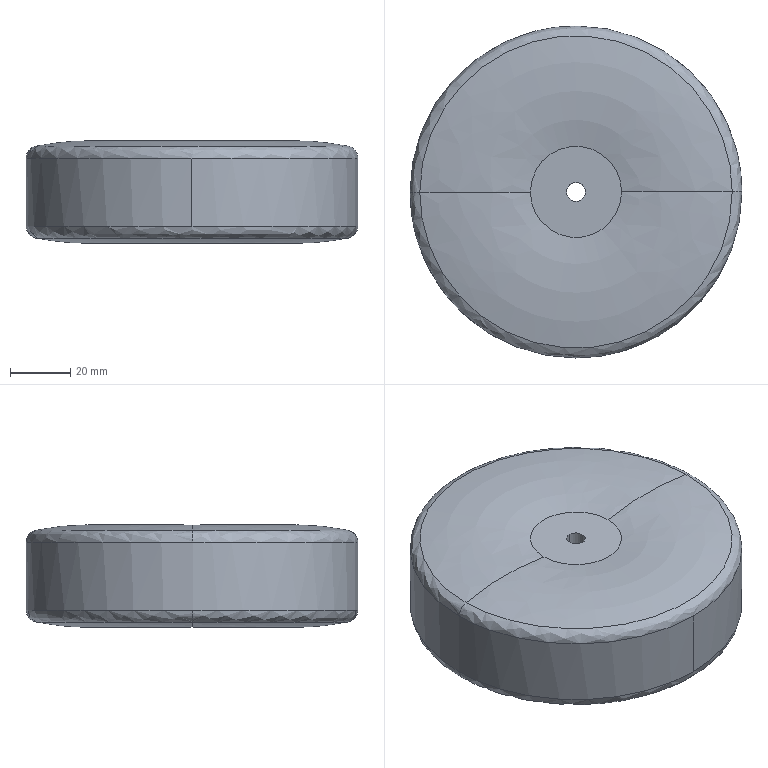Part | SolidWorks | features BaseBody 1 | 1 solid | 19 faces | box 110 x 110 x 34 mm | volume 303850 mm3 | spline 10 | cylinder 6 | plane 3 | commonest cylinder face diameters 6.2 x2 10.5 x2 110 x2
STEP:
#1=CARTESIAN_POINT('',(576.44,-187.714,1.889));
#2=VERTEX_POINT('',#1);
#3=CARTESIAN_POINT('',(606.64,-187.582,1.889));
#4=VERTEX_POINT('',#3);
#5=CARTESIAN_POINT('',(591.54,-187.648,1.889));
#6=DIRECTION('',(0.000000001,-0.000000003,1.));
#7=DIRECTION('',(0.,1.,0.000000003));
#8=AXIS2_PLACEMENT_3D('',#5,#6,#7);
#9=CIRCLE('',#8,15.1);
#10=EDGE_CURVE('',#2,#4,#9,.T.);
#11=ORIENTED_EDGE('',*,*,#10,.F.);
#12=CARTESIAN_POINT('',(539.765,-187.873,1.813));
#13=VERTEX_POINT('',#12);
#14=CARTESIAN_POINT('',(576.44,-187.714,1.889));
#15=CARTESIAN_POINT('',(573.541,-187.726,2.449));
#16=CARTESIAN_POINT('',(567.449,-187.753,3.336));
#17=CARTESIAN_POINT('',(558.099,-187.794,3.786));
#18=CARTESIAN_POINT('',(548.751,-187.834,3.297));
#19=CARTESIAN_POINT('',(542.662,-187.861,2.385));
#20=CARTESIAN_POINT('',(539.765,-187.873,1.813));
#21=B_SPLINE_CURVE_WITH_KNOTS('',3,(#14,#15,#16,#17,#18,#19,#20),.UNSPECIFIED.,.F.,.F.,(4,1,1,1,4),(0.01923,0.25,0.5,0.75,0.9808),.UNSPECIFIED.);
#22=EDGE_CURVE('',#2,#13,#21,.T.);
#23=ORIENTED_EDGE('',*,*,#22,.T.);
#24=CARTESIAN_POINT('',(643.315,-187.423,1.813));
#25=VERTEX_POINT('',#24);
#26=CARTESIAN_POINT('',(643.315,-187.423,1.813));
#27=CARTESIAN_POINT('',(643.765,-290.972,1.813));
#28=CARTESIAN_POINT('',(540.216,-291.423,1.813));
#29=CARTESIAN_POINT('',(539.765,-187.873,1.813));
#30=(BOUNDED_CURVE()B_SPLINE_CURVE(3,(#26,#27,#28,#29),.UNSPECIFIED.,.F.,.F.)B_SPLINE_CURVE_WITH_KNOTS((4,4),(0.,1.),.UNSPECIFIED.)CURVE()GEOMETRIC_REPRESENTATION_ITEM()RATIONAL_B_SPLINE_CURVE((1.,0.3333,0.3333,1.))REPRESENTATION_ITEM(''));
#31=EDGE_CURVE('',#25,#13,#30,.T.);
#32=ORIENTED_EDGE('',*,*,#31,.F.);
#33=CARTESIAN_POINT('',(606.64,-187.582,1.889));
#34=CARTESIAN_POINT('',(609.538,-187.57,2.449));
#35=CARTESIAN_POINT('',(615.631,-187.543,3.336));
#36=CARTESIAN_POINT('',(624.981,-187.503,3.786));
#37=CARTESIAN_POINT('',(634.329,-187.462,3.297));
#38=CARTESIAN_POINT('',(640.418,-187.435,2.385));
#39=CARTESIAN_POINT('',(643.315,-187.423,1.813));
#40=B_SPLINE_CURVE_WITH_KNOTS('',3,(#33,#34,#35,#36,#37,#38,#39),.UNSPECIFIED.,.F.,.F.,(4,1,1,1,4),(0.01923,0.25,0.5,0.75,0.9808),.UNSPECIFIED.);
#41=EDGE_CURVE('',#4,#25,#40,.T.);
#42=ORIENTED_EDGE('',*,*,#41,.F.);
#43=EDGE_LOOP('',(#11,#23,#32,#42));
#44=FACE_OUTER_BOUND('',#43,.T.);
#45=CARTESIAN_POINT('',(606.64,-187.582,1.889));
#46=CARTESIAN_POINT('',(606.771,-217.782,1.889));
#47=CARTESIAN_POINT('',(576.572,-217.914,1.889));
#48=CARTESIAN_POINT('',(576.44,-187.714,1.889));
#49=CARTESIAN_POINT('',(609.538,-187.57,2.449));
#50=CARTESIAN_POINT('',(609.695,-223.567,2.449));
#51=CARTESIAN_POINT('',(573.698,-223.724,2.449));
#52=CARTESIAN_POINT('',(573.541,-187.726,2.449));
#53=CARTESIAN_POINT('',(615.631,-187.543,3.336));
#54=CARTESIAN_POINT('',(615.841,-235.726,3.336));
#55=CARTESIAN_POINT('',(567.658,-235.936,3.336));
#56=CARTESIAN_POINT('',(567.449,-187.753,3.336));
#57=CARTESIAN_POINT('',(624.981,-187.503,3.786));
#58=CARTESIAN_POINT('',(625.272,-254.385,3.786));
#59=CARTESIAN_POINT('',(558.39,-254.676,3.786));
#60=CARTESIAN_POINT('',(558.099,-187.794,3.786));
#61=CARTESIAN_POINT('',(634.329,-187.462,3.297));
#62=CARTESIAN_POINT('',(634.702,-273.04,3.297));
#63=CARTESIAN_POINT('',(549.123,-273.413,3.297));
#64=CARTESIAN_POINT('',(548.751,-187.834,3.297));
#65=CARTESIAN_POINT('',(640.418,-187.435,2.385));
#66=CARTESIAN_POINT('',(640.844,-285.192,2.385));
#67=CARTESIAN_POINT('',(543.087,-285.618,2.385));
#68=CARTESIAN_POINT('',(542.662,-187.861,2.385));
#69=CARTESIAN_POINT('',(643.315,-187.423,1.813));
#70=CARTESIAN_POINT('',(643.765,-290.972,1.813));
#71=CARTESIAN_POINT('',(540.216,-291.423,1.813));
#72=CARTESIAN_POINT('',(539.765,-187.873,1.813));
#73=(BOUNDED_SURFACE()B_SPLINE_SURFACE(3,3,((#45,#46,#47,#48),(#49,#50,#51,#52),(#53,#54,#55,#56),(#57,#58,#59,#60),(#61,#62,#63,#64),(#65,#66,#67,#68),(#69,#70,#71,#72)),.UNSPECIFIED.,.F.,.F.,.F.)B_SPLINE_SURFACE_WITH_KNOTS((4,1,1,1,4),(4,4),(0.01923,0.25,0.5,0.75,0.9808),(0.,1.),.UNSPECIFIED.)GEOMETRIC_REPRESENTATION_ITEM()RATIONAL_B_SPLINE_SURFACE(((1.,0.3333,0.3333,1.),(1.,0.3333,0.3333,1.),(1.,0.3333,0.3333,1.),(1.,0.3333,0.3333,1.),(1.,0.3333,0.3333,1.),(1.,0.3333,0.3333,1.),(1.,0.3333,0.3333,1.)))REPRESENTATION_ITEM('')SURFACE());
#74=ADVANCED_FACE('',(#44),#73,.F.);
#75=ORIENTED_EDGE('',*,*,#31,.T.);
#76=CARTESIAN_POINT('',(536.541,-187.888,-2.111));
#77=VERTEX_POINT('',#76);
#78=CARTESIAN_POINT('',(539.765,-187.873,1.813));
#79=CARTESIAN_POINT('',(539.333,-187.875,1.727));
#80=CARTESIAN_POINT('',(538.463,-187.879,1.4));
#81=CARTESIAN_POINT('',(537.383,-187.884,0.4829));
#82=CARTESIAN_POINT('',(536.693,-187.887,-0.7541));
#83=CARTESIAN_POINT('',(536.541,-187.888,-1.671));
#84=CARTESIAN_POINT('',(536.541,-187.888,-2.111));
#85=B_SPLINE_CURVE_WITH_KNOTS('',3,(#78,#79,#80,#81,#82,#83,#84),.UNSPECIFIED.,.F.,.F.,(4,1,1,1,4),(0.01923,0.25,0.5,0.75,0.9808),.UNSPECIFIED.);
#86=EDGE_CURVE('',#13,#77,#85,.T.);
#87=ORIENTED_EDGE('',*,*,#86,.T.);
#88=CARTESIAN_POINT('',(591.54,-242.648,-2.111));
#89=VERTEX_POINT('',#88);
#90=CARTESIAN_POINT('',(591.54,-242.648,-2.111));
#91=CARTESIAN_POINT('',(587.95,-242.648,-2.111));
#92=CARTESIAN_POINT('',(584.361,-242.296,-2.111));
#93=CARTESIAN_POINT('',(577.318,-240.899,-2.111));
#94=CARTESIAN_POINT('',(573.866,-239.855,-2.111));
#95=CARTESIAN_POINT('',(567.23,-237.114,-2.111));
#96=CARTESIAN_POINT('',(564.046,-235.418,-2.111));
#97=CARTESIAN_POINT('',(558.07,-231.439,-2.111));
#98=CARTESIAN_POINT('',(555.278,-229.156,-2.111));
#99=CARTESIAN_POINT('',(550.19,-224.091,-2.111));
#100=CARTESIAN_POINT('',(547.895,-221.308,-2.111));
#101=CARTESIAN_POINT('',(543.89,-215.349,-2.111));
#102=CARTESIAN_POINT('',(542.18,-212.173,-2.111));
#103=CARTESIAN_POINT('',(539.411,-205.549,-2.111));
#104=CARTESIAN_POINT('',(538.352,-202.102,-2.111));
#105=CARTESIAN_POINT('',(536.924,-195.065,-2.111));
#106=CARTESIAN_POINT('',(536.556,-191.477,-2.111));
#107=CARTESIAN_POINT('',(536.541,-187.888,-2.111));
#108=B_SPLINE_CURVE_WITH_KNOTS('',3,(#90,#91,#92,#93,#94,#95,#96,#97,#98,#99,#100,#101,#102,#103,#104,#105,#106,#107),.UNSPECIFIED.,.F.,.F.,(4,2,2,2,2,2,2,2,4),(0.5014,0.5637,0.626,0.6884,0.7507,0.813,0.8753,0.9377,1.),.UNSPECIFIED.);
#109=EDGE_CURVE('',#89,#77,#108,.T.);
#110=ORIENTED_EDGE('',*,*,#109,.F.);
#111=CARTESIAN_POINT('',(646.539,-187.409,-2.111));
#112=VERTEX_POINT('',#111);
#113=CARTESIAN_POINT('',(646.539,-187.409,-2.111));
#114=CARTESIAN_POINT('',(646.555,-191.018,-2.111));
#115=CARTESIAN_POINT('',(646.214,-194.63,-2.111));
#116=CARTESIAN_POINT('',(644.833,-201.716,-2.111));
#117=CARTESIAN_POINT('',(643.792,-205.19,-2.111));
#118=CARTESIAN_POINT('',(641.051,-211.869,-2.111));
#119=CARTESIAN_POINT('',(639.351,-215.073,-2.111));
#120=CARTESIAN_POINT('',(635.356,-221.087,-2.111));
#121=CARTESIAN_POINT('',(633.062,-223.896,-2.111));
#122=CARTESIAN_POINT('',(627.968,-229.012,-2.111));
#123=CARTESIAN_POINT('',(625.169,-231.319,-2.111));
#124=CARTESIAN_POINT('',(619.173,-235.339,-2.111));
#125=CARTESIAN_POINT('',(615.976,-237.054,-2.111));
#126=CARTESIAN_POINT('',(609.309,-239.824,-2.111));
#127=CARTESIAN_POINT('',(605.839,-240.879,-2.111));
#128=CARTESIAN_POINT('',(598.759,-242.292,-2.111));
#129=CARTESIAN_POINT('',(595.15,-242.648,-2.111));
#130=CARTESIAN_POINT('',(591.54,-242.648,-2.111));
#131=B_SPLINE_CURVE_WITH_KNOTS('',3,(#113,#114,#115,#116,#117,#118,#119,#120,#121,#122,#123,#124,#125,#126,#127,#128,#129,#130),.UNSPECIFIED.,.F.,.F.,(4,2,2,2,2,2,2,2,4),(0.,0.06267,0.1253,0.188,0.2507,0.3134,0.376,0.4387,0.5014),.UNSPECIFIED.);
#132=EDGE_CURVE('',#112,#89,#131,.T.);
#133=ORIENTED_EDGE('',*,*,#132,.F.);
#134=CARTESIAN_POINT('',(643.315,-187.423,1.813));
#135=CARTESIAN_POINT('',(643.747,-187.421,1.727));
#136=CARTESIAN_POINT('',(644.617,-187.417,1.4));
#137=CARTESIAN_POINT('',(645.696,-187.412,0.4829));
#138=CARTESIAN_POINT('',(646.387,-187.409,-0.7541));
#139=CARTESIAN_POINT('',(646.539,-187.409,-1.671));
#140=CARTESIAN_POINT('',(646.539,-187.409,-2.111));
#141=B_SPLINE_CURVE_WITH_KNOTS('',3,(#134,#135,#136,#137,#138,#139,#140),.UNSPECIFIED.,.F.,.F.,(4,1,1,1,4),(0.01923,0.25,0.5,0.75,0.9808),.UNSPECIFIED.);
#142=EDGE_CURVE('',#25,#112,#141,.T.);
#143=ORIENTED_EDGE('',*,*,#142,.F.);
#144=EDGE_LOOP('',(#75,#87,#110,#133,#143));
#145=FACE_OUTER_BOUND('',#144,.T.);
#146=CARTESIAN_POINT('',(643.315,-187.423,1.813));
#147=CARTESIAN_POINT('',(643.765,-290.972,1.813));
#148=CARTESIAN_POINT('',(540.216,-291.423,1.813));
#149=CARTESIAN_POINT('',(539.765,-187.873,1.813));
#150=CARTESIAN_POINT('',(643.747,-187.421,1.727));
#151=CARTESIAN_POINT('',(644.201,-291.834,1.727));
#152=CARTESIAN_POINT('',(539.788,-292.289,1.727));
#153=CARTESIAN_POINT('',(539.333,-187.875,1.727));
#154=CARTESIAN_POINT('',(644.617,-187.417,1.4));
#155=CARTESIAN_POINT('',(645.079,-293.571,1.4));
#156=CARTESIAN_POINT('',(538.925,-294.033,1.4));
#157=CARTESIAN_POINT('',(538.463,-187.879,1.4));
#158=CARTESIAN_POINT('',(645.696,-187.412,0.4829));
#159=CARTESIAN_POINT('',(646.168,-295.725,0.4829));
#160=CARTESIAN_POINT('',(537.855,-296.197,0.4829));
#161=CARTESIAN_POINT('',(537.383,-187.884,0.4829));
#162=CARTESIAN_POINT('',(646.387,-187.409,-0.7541));
#163=CARTESIAN_POINT('',(646.864,-297.103,-0.7541));
#164=CARTESIAN_POINT('',(537.171,-297.58,-0.7541));
#165=CARTESIAN_POINT('',(536.693,-187.887,-0.7541));
#166=CARTESIAN_POINT('',(646.539,-187.409,-1.671));
#167=CARTESIAN_POINT('',(647.018,-297.408,-1.671));
#168=CARTESIAN_POINT('',(537.019,-297.886,-1.671));
#169=CARTESIAN_POINT('',(536.541,-187.888,-1.671));
#170=CARTESIAN_POINT('',(646.539,-187.409,-2.111));
#171=CARTESIAN_POINT('',(647.018,-297.408,-2.111));
#172=CARTESIAN_POINT('',(537.019,-297.886,-2.111));
#173=CARTESIAN_POINT('',(536.541,-187.888,-2.111));
#174=(BOUNDED_SURFACE()B_SPLINE_SURFACE(3,3,((#146,#147,#148,#149),(#150,#151,#152,#153),(#154,#155,#156,#157),(#158,#159,#160,#161),(#162,#163,#164,#165),(#166,#167,#168,#169),(#170,#171,#172,#173)),.UNSPECIFIED.,.F.,.F.,.T.)B_SPLINE_SURFACE_WITH_KNOTS((4,1,1,1,4),(4,4),(0.01923,0.25,0.5,0.75,0.9808),(0.,1.),.UNSPECIFIED.)GEOMETRIC_REPRESENTATION_ITEM()RATIONAL_B_SPLINE_SURFACE(((1.,0.3333,0.3333,1.),(1.,0.3333,0.3333,1.),(1.,0.3333,0.3333,1.),(1.,0.3333,0.3333,1.),(1.,0.3333,0.3333,1.),(1.,0.3333,0.3333,1.),(1.,0.3333,0.3333,1.)))REPRESENTATION_ITEM('')SURFACE());
#175=ADVANCED_FACE('',(#145),#174,.F.);
#176=CARTESIAN_POINT('',(591.54,-242.648,-24.711));
#177=VERTEX_POINT('',#176);
#178=CARTESIAN_POINT('',(536.541,-187.888,-24.711));
#179=VERTEX_POINT('',#178);
#180=CARTESIAN_POINT('',(591.54,-242.648,-24.711));
#181=CARTESIAN_POINT('',(559.433,-242.648,-24.711));
#182=CARTESIAN_POINT('',(536.68,-219.994,-24.711));
#183=CARTESIAN_POINT('',(536.541,-187.888,-24.711));
#184=(BOUNDED_CURVE()B_SPLINE_CURVE(3,(#180,#181,#182,#183),.UNSPECIFIED.,.F.,.F.)B_SPLINE_CURVE_WITH_KNOTS((4,4),(0.5014,1.),.UNSPECIFIED.)CURVE()GEOMETRIC_REPRESENTATION_ITEM()RATIONAL_B_SPLINE_CURVE((1.,0.8058,0.8058,1.))REPRESENTATION_ITEM(''));
#185=EDGE_CURVE('',#177,#179,#184,.T.);
#186=ORIENTED_EDGE('',*,*,#185,.T.);
#187=CARTESIAN_POINT('',(539.782,-187.873,-28.639));
#188=VERTEX_POINT('',#187);
#189=CARTESIAN_POINT('',(536.541,-187.888,-24.711));
#190=CARTESIAN_POINT('',(536.541,-187.888,-25.153));
#191=CARTESIAN_POINT('',(536.694,-187.887,-26.073));
#192=CARTESIAN_POINT('',(537.389,-187.884,-27.313));
#193=CARTESIAN_POINT('',(538.474,-187.879,-28.23));
#194=CARTESIAN_POINT('',(539.348,-187.875,-28.555));
#195=CARTESIAN_POINT('',(539.782,-187.873,-28.639));
#196=B_SPLINE_CURVE_WITH_KNOTS('',3,(#189,#190,#191,#192,#193,#194,#195),.UNSPECIFIED.,.F.,.F.,(4,1,1,1,4),(0.01923,0.25,0.5,0.75,0.9808),.UNSPECIFIED.);
#197=EDGE_CURVE('',#179,#188,#196,.T.);
#198=ORIENTED_EDGE('',*,*,#197,.T.);
#199=CARTESIAN_POINT('',(643.298,-187.423,-28.639));
#200=VERTEX_POINT('',#199);
#201=CARTESIAN_POINT('',(643.298,-187.423,-28.639));
#202=CARTESIAN_POINT('',(643.749,-290.939,-28.639));
#203=CARTESIAN_POINT('',(540.232,-291.39,-28.639));
#204=CARTESIAN_POINT('',(539.782,-187.873,-28.639));
#205=(BOUNDED_CURVE()B_SPLINE_CURVE(3,(#201,#202,#203,#204),.UNSPECIFIED.,.F.,.F.)B_SPLINE_CURVE_WITH_KNOTS((4,4),(0.,1.),.UNSPECIFIED.)CURVE()GEOMETRIC_REPRESENTATION_ITEM()RATIONAL_B_SPLINE_CURVE((1.,0.3333,0.3333,1.))REPRESENTATION_ITEM(''));
#206=EDGE_CURVE('',#200,#188,#205,.T.);
#207=ORIENTED_EDGE('',*,*,#206,.F.);
#208=CARTESIAN_POINT('',(646.539,-187.409,-24.711));
#209=VERTEX_POINT('',#208);
#210=CARTESIAN_POINT('',(646.539,-187.409,-24.711));
#211=CARTESIAN_POINT('',(646.539,-187.409,-25.153));
#212=CARTESIAN_POINT('',(646.386,-187.409,-26.073));
#213=CARTESIAN_POINT('',(645.691,-187.412,-27.313));
#214=CARTESIAN_POINT('',(644.606,-187.417,-28.23));
#215=CARTESIAN_POINT('',(643.732,-187.421,-28.555));
#216=CARTESIAN_POINT('',(643.298,-187.423,-28.639));
#217=B_SPLINE_CURVE_WITH_KNOTS('',3,(#210,#211,#212,#213,#214,#215,#216),.UNSPECIFIED.,.F.,.F.,(4,1,1,1,4),(0.01923,0.25,0.5,0.75,0.9808),.UNSPECIFIED.);
#218=EDGE_CURVE('',#209,#200,#217,.T.);
#219=ORIENTED_EDGE('',*,*,#218,.F.);
#220=CARTESIAN_POINT('',(646.539,-187.409,-24.711));
#221=CARTESIAN_POINT('',(646.68,-219.738,-24.711));
#222=CARTESIAN_POINT('',(623.87,-242.648,-24.711));
#223=CARTESIAN_POINT('',(591.54,-242.648,-24.711));
#224=(BOUNDED_CURVE()B_SPLINE_CURVE(3,(#220,#221,#222,#223),.UNSPECIFIED.,.F.,.F.)B_SPLINE_CURVE_WITH_KNOTS((4,4),(0.,0.5014),.UNSPECIFIED.)CURVE()GEOMETRIC_REPRESENTATION_ITEM()RATIONAL_B_SPLINE_CURVE((1.,0.8037,0.8037,1.))REPRESENTATION_ITEM(''));
#225=EDGE_CURVE('',#209,#177,#224,.T.);
#226=ORIENTED_EDGE('',*,*,#225,.T.);
#227=EDGE_LOOP('',(#186,#198,#207,#219,#226));
#228=FACE_OUTER_BOUND('',#227,.T.);
#229=CARTESIAN_POINT('',(646.539,-187.409,-24.711));
#230=CARTESIAN_POINT('',(647.018,-297.408,-24.711));
#231=CARTESIAN_POINT('',(537.019,-297.886,-24.711));
#232=CARTESIAN_POINT('',(536.541,-187.888,-24.711));
#233=CARTESIAN_POINT('',(646.539,-187.409,-25.153));
#234=CARTESIAN_POINT('',(647.018,-297.408,-25.153));
#235=CARTESIAN_POINT('',(537.019,-297.886,-25.153));
#236=CARTESIAN_POINT('',(536.541,-187.888,-25.153));
#237=CARTESIAN_POINT('',(646.386,-187.409,-26.073));
#238=CARTESIAN_POINT('',(646.863,-297.101,-26.073));
#239=CARTESIAN_POINT('',(537.172,-297.579,-26.073));
#240=CARTESIAN_POINT('',(536.694,-187.887,-26.073));
#241=CARTESIAN_POINT('',(645.691,-187.412,-27.313));
#242=CARTESIAN_POINT('',(646.163,-295.715,-27.313));
#243=CARTESIAN_POINT('',(537.86,-296.187,-27.313));
#244=CARTESIAN_POINT('',(537.389,-187.884,-27.313));
#245=CARTESIAN_POINT('',(644.606,-187.417,-28.23));
#246=CARTESIAN_POINT('',(645.068,-293.549,-28.23));
#247=CARTESIAN_POINT('',(538.936,-294.011,-28.23));
#248=CARTESIAN_POINT('',(538.474,-187.879,-28.23));
#249=CARTESIAN_POINT('',(643.732,-187.421,-28.555));
#250=CARTESIAN_POINT('',(644.186,-291.804,-28.555));
#251=CARTESIAN_POINT('',(539.803,-292.259,-28.555));
#252=CARTESIAN_POINT('',(539.348,-187.875,-28.555));
#253=CARTESIAN_POINT('',(643.298,-187.423,-28.639));
#254=CARTESIAN_POINT('',(643.749,-290.939,-28.639));
#255=CARTESIAN_POINT('',(540.232,-291.39,-28.639));
#256=CARTESIAN_POINT('',(539.782,-187.873,-28.639));
#257=(BOUNDED_SURFACE()B_SPLINE_SURFACE(3,3,((#229,#230,#231,#232),(#233,#234,#235,#236),(#237,#238,#239,#240),(#241,#242,#243,#244),(#245,#246,#247,#248),(#249,#250,#251,#252),(#253,#254,#255,#256)),.UNSPECIFIED.,.F.,.F.,.F.)B_SPLINE_SURFACE_WITH_KNOTS((4,1,1,1,4),(4,4),(0.01923,0.25,0.5,0.75,0.9808),(0.,1.),.UNSPECIFIED.)GEOMETRIC_REPRESENTATION_ITEM()RATIONAL_B_SPLINE_SURFACE(((1.,0.3333,0.3333,1.),(1.,0.3333,0.3333,1.),(1.,0.3333,0.3333,1.),(1.,0.3333,0.3333,1.),(1.,0.3333,0.3333,1.),(1.,0.3333,0.3333,1.),(1.,0.3333,0.3333,1.)))REPRESENTATION_ITEM('')SURFACE());
#258=ADVANCED_FACE('',(#228),#257,.F.);
#259=ORIENTED_EDGE('',*,*,#206,.T.);
#260=CARTESIAN_POINT('',(574.039,-187.724,-29.005));
#261=VERTEX_POINT('',#260);
#262=CARTESIAN_POINT('',(539.782,-187.873,-28.639));
#263=CARTESIAN_POINT('',(542.487,-187.862,-29.161));
#264=CARTESIAN_POINT('',(548.171,-187.837,-30.006));
#265=CARTESIAN_POINT('',(556.892,-187.799,-30.509));
#266=CARTESIAN_POINT('',(565.622,-187.761,-30.193));
#267=CARTESIAN_POINT('',(571.323,-187.736,-29.47));
#268=CARTESIAN_POINT('',(574.039,-187.724,-29.005));
#269=B_SPLINE_CURVE_WITH_KNOTS('',3,(#262,#263,#264,#265,#266,#267,#268),.UNSPECIFIED.,.F.,.F.,(4,1,1,1,4),(0.01923,0.25,0.5,0.75,0.9808),.UNSPECIFIED.);
#270=EDGE_CURVE('',#188,#261,#269,.T.);
#271=ORIENTED_EDGE('',*,*,#270,.T.);
#272=CARTESIAN_POINT('',(609.041,-187.572,-29.005));
#273=VERTEX_POINT('',#272);
#274=CARTESIAN_POINT('',(591.54,-187.648,-29.005));
#275=DIRECTION('',(-0.000000001,0.000000003,-1.));
#276=DIRECTION('',(1.,0.004352,-0.000000001));
#277=AXIS2_PLACEMENT_3D('',#274,#275,#276);
#278=CIRCLE('',#277,17.501);
#279=EDGE_CURVE('',#273,#261,#278,.T.);
#280=ORIENTED_EDGE('',*,*,#279,.F.);
#281=CARTESIAN_POINT('',(643.298,-187.423,-28.639));
#282=CARTESIAN_POINT('',(640.593,-187.435,-29.161));
#283=CARTESIAN_POINT('',(634.909,-187.459,-30.006));
#284=CARTESIAN_POINT('',(626.187,-187.497,-30.509));
#285=CARTESIAN_POINT('',(617.457,-187.535,-30.193));
#286=CARTESIAN_POINT('',(611.757,-187.56,-29.47));
#287=CARTESIAN_POINT('',(609.041,-187.572,-29.005));
#288=B_SPLINE_CURVE_WITH_KNOTS('',3,(#281,#282,#283,#284,#285,#286,#287),.UNSPECIFIED.,.F.,.F.,(4,1,1,1,4),(0.01923,0.25,0.5,0.75,0.9808),.UNSPECIFIED.);
#289=EDGE_CURVE('',#200,#273,#288,.T.);
#290=ORIENTED_EDGE('',*,*,#289,.F.);
#291=EDGE_LOOP('',(#259,#271,#280,#290));
#292=FACE_OUTER_BOUND('',#291,.T.);
#293=CARTESIAN_POINT('',(643.298,-187.423,-28.639));
#294=CARTESIAN_POINT('',(643.749,-290.939,-28.639));
#295=CARTESIAN_POINT('',(540.232,-291.39,-28.639));
#296=CARTESIAN_POINT('',(539.782,-187.873,-28.639));
#297=CARTESIAN_POINT('',(640.593,-187.435,-29.161));
#298=CARTESIAN_POINT('',(641.019,-285.54,-29.161));
#299=CARTESIAN_POINT('',(542.914,-285.967,-29.161));
#300=CARTESIAN_POINT('',(542.487,-187.862,-29.161));
#301=CARTESIAN_POINT('',(634.909,-187.459,-30.006));
#302=CARTESIAN_POINT('',(635.286,-274.197,-30.006));
#303=CARTESIAN_POINT('',(548.549,-274.574,-30.006));
#304=CARTESIAN_POINT('',(548.171,-187.837,-30.006));
#305=CARTESIAN_POINT('',(626.187,-187.497,-30.509));
#306=CARTESIAN_POINT('',(626.489,-256.792,-30.509));
#307=CARTESIAN_POINT('',(557.194,-257.094,-30.509));
#308=CARTESIAN_POINT('',(556.892,-187.799,-30.509));
#309=CARTESIAN_POINT('',(617.457,-187.535,-30.193));
#310=CARTESIAN_POINT('',(617.683,-239.37,-30.193));
#311=CARTESIAN_POINT('',(565.848,-239.596,-30.193));
#312=CARTESIAN_POINT('',(565.622,-187.761,-30.193));
#313=CARTESIAN_POINT('',(611.757,-187.56,-29.47));
#314=CARTESIAN_POINT('',(611.933,-227.994,-29.47));
#315=CARTESIAN_POINT('',(571.499,-228.17,-29.47));
#316=CARTESIAN_POINT('',(571.323,-187.736,-29.47));
#317=CARTESIAN_POINT('',(609.041,-187.572,-29.005));
#318=CARTESIAN_POINT('',(609.193,-222.574,-29.005));
#319=CARTESIAN_POINT('',(574.192,-222.726,-29.005));
#320=CARTESIAN_POINT('',(574.039,-187.724,-29.005));
#321=(BOUNDED_SURFACE()B_SPLINE_SURFACE(3,3,((#293,#294,#295,#296),(#297,#298,#299,#300),(#301,#302,#303,#304),(#305,#306,#307,#308),(#309,#310,#311,#312),(#313,#314,#315,#316),(#317,#318,#319,#320)),.UNSPECIFIED.,.F.,.F.,.T.)B_SPLINE_SURFACE_WITH_KNOTS((4,1,1,1,4),(4,4),(0.01923,0.25,0.5,0.75,0.9808),(0.,1.),.UNSPECIFIED.)GEOMETRIC_REPRESENTATION_ITEM()RATIONAL_B_SPLINE_SURFACE(((1.,0.3333,0.3333,1.),(1.,0.3333,0.3333,1.),(1.,0.3333,0.3333,1.),(1.,0.3333,0.3333,1.),(1.,0.3333,0.3333,1.),(1.,0.3333,0.3333,1.),(1.,0.3333,0.3333,1.)))REPRESENTATION_ITEM('')SURFACE());
#322=ADVANCED_FACE('',(#292),#321,.F.);
#323=ORIENTED_EDGE('',*,*,#279,.T.);
#324=CARTESIAN_POINT('',(575.79,-187.717,-28.111));
#325=VERTEX_POINT('',#324);
#326=CARTESIAN_POINT('',(574.039,-187.724,-29.005));
#327=CARTESIAN_POINT('',(574.367,-187.723,-28.949));
#328=CARTESIAN_POINT('',(575.006,-187.72,-28.737));
#329=CARTESIAN_POINT('',(575.552,-187.718,-28.344));
#330=CARTESIAN_POINT('',(575.79,-187.717,-28.111));
#331=B_SPLINE_CURVE_WITH_KNOTS('',3,(#326,#327,#328,#329,#330),.UNSPECIFIED.,.F.,.F.,(4,1,4),(0.01923,0.5,0.9808),.UNSPECIFIED.);
#332=EDGE_CURVE('',#261,#325,#331,.T.);
#333=ORIENTED_EDGE('',*,*,#332,.T.);
#334=CARTESIAN_POINT('',(607.29,-187.58,-28.111));
#335=VERTEX_POINT('',#334);
#336=CARTESIAN_POINT('',(591.54,-187.648,-28.111));
#337=DIRECTION('',(-0.000000001,0.000000003,-1.));
#338=DIRECTION('',(0.,1.,0.000000003));
#339=AXIS2_PLACEMENT_3D('',#336,#337,#338);
#340=CIRCLE('',#339,15.75);
#341=EDGE_CURVE('',#335,#325,#340,.T.);
#342=ORIENTED_EDGE('',*,*,#341,.F.);
#343=CARTESIAN_POINT('',(609.041,-187.572,-29.005));
#344=CARTESIAN_POINT('',(608.713,-187.573,-28.949));
#345=CARTESIAN_POINT('',(608.074,-187.576,-28.737));
#346=CARTESIAN_POINT('',(607.528,-187.579,-28.344));
#347=CARTESIAN_POINT('',(607.29,-187.58,-28.111));
#348=B_SPLINE_CURVE_WITH_KNOTS('',3,(#343,#344,#345,#346,#347),.UNSPECIFIED.,.F.,.F.,(4,1,4),(0.01923,0.5,0.9808),.UNSPECIFIED.);
#349=EDGE_CURVE('',#273,#335,#348,.T.);
#350=ORIENTED_EDGE('',*,*,#349,.F.);
#351=EDGE_LOOP('',(#323,#333,#342,#350));
#352=FACE_OUTER_BOUND('',#351,.T.);
#353=CARTESIAN_POINT('',(609.041,-187.572,-29.005));
#354=CARTESIAN_POINT('',(609.193,-222.574,-29.005));
#355=CARTESIAN_POINT('',(574.192,-222.726,-29.005));
#356=CARTESIAN_POINT('',(574.039,-187.724,-29.005));
#357=CARTESIAN_POINT('',(608.713,-187.573,-28.949));
#358=CARTESIAN_POINT('',(608.862,-221.919,-28.949));
#359=CARTESIAN_POINT('',(574.517,-222.069,-28.949));
#360=CARTESIAN_POINT('',(574.367,-187.723,-28.949));
#361=CARTESIAN_POINT('',(608.074,-187.576,-28.737));
#362=CARTESIAN_POINT('',(608.218,-220.645,-28.737));
#363=CARTESIAN_POINT('',(575.15,-220.788,-28.737));
#364=CARTESIAN_POINT('',(575.006,-187.72,-28.737));
#365=CARTESIAN_POINT('',(607.528,-187.579,-28.344));
#366=CARTESIAN_POINT('',(607.667,-219.554,-28.344));
#367=CARTESIAN_POINT('',(575.691,-219.693,-28.344));
#368=CARTESIAN_POINT('',(575.552,-187.718,-28.344));
#369=CARTESIAN_POINT('',(607.29,-187.58,-28.111));
#370=CARTESIAN_POINT('',(607.427,-219.079,-28.111));
#371=CARTESIAN_POINT('',(575.927,-219.216,-28.111));
#372=CARTESIAN_POINT('',(575.79,-187.717,-28.111));
#373=(BOUNDED_SURFACE()B_SPLINE_SURFACE(3,3,((#353,#354,#355,#356),(#357,#358,#359,#360),(#361,#362,#363,#364),(#365,#366,#367,#368),(#369,#370,#371,#372)),.UNSPECIFIED.,.F.,.F.,.T.)B_SPLINE_SURFACE_WITH_KNOTS((4,1,4),(4,4),(0.01923,0.5,0.9808),(0.,1.),.UNSPECIFIED.)GEOMETRIC_REPRESENTATION_ITEM()RATIONAL_B_SPLINE_SURFACE(((1.,0.3333,0.3333,1.),(1.,0.3333,0.3333,1.),(1.,0.3333,0.3333,1.),(1.,0.3333,0.3333,1.),(1.,0.3333,0.3333,1.)))REPRESENTATION_ITEM('')SURFACE());
#374=ADVANCED_FACE('',(#352),#373,.F.);
#375=CARTESIAN_POINT('',(591.54,-184.548,1.889));
#376=VERTEX_POINT('',#375);
#377=CARTESIAN_POINT('',(591.54,-190.748,1.889));
#378=VERTEX_POINT('',#377);
#379=CARTESIAN_POINT('',(591.54,-187.648,1.889));
#380=DIRECTION('',(0.000000001,-0.000000003,1.));
#381=DIRECTION('',(0.,1.,0.000000003));
#382=AXIS2_PLACEMENT_3D('',#379,#380,#381);
#383=CIRCLE('',#382,3.1);
#384=EDGE_CURVE('',#376,#378,#383,.T.);
#385=ORIENTED_EDGE('',*,*,#384,.T.);
#386=CARTESIAN_POINT('',(591.54,-190.748,-22.111));
#387=VERTEX_POINT('',#386);
#388=CARTESIAN_POINT('',(591.54,-190.748,1.889));
#389=DIRECTION('',(-0.000000001,0.000000003,-1.));
#390=VECTOR('',#389,1000.);
#391=LINE('',#388,#390);
#392=EDGE_CURVE('',#378,#387,#391,.T.);
#393=ORIENTED_EDGE('',*,*,#392,.T.);
#394=CARTESIAN_POINT('',(591.54,-184.548,-22.111));
#395=VERTEX_POINT('',#394);
#396=CARTESIAN_POINT('',(591.54,-187.648,-22.111));
#397=DIRECTION('',(-0.000000001,0.000000003,-1.));
#398=DIRECTION('',(0.,1.,0.000000003));
#399=AXIS2_PLACEMENT_3D('',#396,#397,#398);
#400=CIRCLE('',#399,3.1);
#401=EDGE_CURVE('',#387,#395,#400,.T.);
#402=ORIENTED_EDGE('',*,*,#401,.T.);
#403=CARTESIAN_POINT('',(591.54,-184.548,1.889));
#404=DIRECTION('',(-0.000000001,0.000000003,-1.));
#405=VECTOR('',#404,1000.);
#406=LINE('',#403,#405);
#407=EDGE_CURVE('',#376,#395,#406,.T.);
#408=ORIENTED_EDGE('',*,*,#407,.F.);
#409=EDGE_LOOP('',(#385,#393,#402,#408));
#410=FACE_OUTER_BOUND('',#409,.T.);
#411=CARTESIAN_POINT('',(591.54,-187.648,1.889));
#412=DIRECTION('',(-0.000000001,0.000000003,-1.));
#413=DIRECTION('',(0.,1.,0.000000003));
#414=AXIS2_PLACEMENT_3D('',#411,#412,#413);
#415=CYLINDRICAL_SURFACE('',#414,3.1);
#416=ADVANCED_FACE('',(#410),#415,.F.);
#417=ORIENTED_EDGE('',*,*,#132,.T.);
#418=CARTESIAN_POINT('',(591.54,-242.648,-2.111));
#419=DIRECTION('',(-0.000000001,0.000000003,-1.));
#420=VECTOR('',#419,1000.);
#421=LINE('',#418,#420);
#422=EDGE_CURVE('',#89,#177,#421,.T.);
#423=ORIENTED_EDGE('',*,*,#422,.T.);
#424=ORIENTED_EDGE('',*,*,#225,.F.);
#425=CARTESIAN_POINT('',(591.54,-132.648,-24.711));
#426=VERTEX_POINT('',#425);
#427=CARTESIAN_POINT('',(591.54,-132.648,-24.711));
#428=CARTESIAN_POINT('',(623.647,-132.648,-24.711));
#429=CARTESIAN_POINT('',(646.4,-155.302,-24.711));
#430=CARTESIAN_POINT('',(646.539,-187.409,-24.711));
#431=(BOUNDED_CURVE()B_SPLINE_CURVE(3,(#427,#428,#429,#430),.UNSPECIFIED.,.F.,.F.)B_SPLINE_CURVE_WITH_KNOTS((4,4),(0.5014,1.),.UNSPECIFIED.)CURVE()GEOMETRIC_REPRESENTATION_ITEM()RATIONAL_B_SPLINE_CURVE((1.,0.8058,0.8058,1.))REPRESENTATION_ITEM(''));
#432=EDGE_CURVE('',#426,#209,#431,.T.);
#433=ORIENTED_EDGE('',*,*,#432,.F.);
#434=CARTESIAN_POINT('',(591.54,-132.648,-2.111));
#435=VERTEX_POINT('',#434);
#436=CARTESIAN_POINT('',(591.54,-132.648,-2.111));
#437=DIRECTION('',(-0.000000001,0.000000003,-1.));
#438=VECTOR('',#437,1000.);
#439=LINE('',#436,#438);
#440=EDGE_CURVE('',#435,#426,#439,.T.);
#441=ORIENTED_EDGE('',*,*,#440,.F.);
#442=CARTESIAN_POINT('',(591.54,-132.648,-2.111));
#443=CARTESIAN_POINT('',(595.13,-132.648,-2.111));
#444=CARTESIAN_POINT('',(598.719,-133.001,-2.111));
#445=CARTESIAN_POINT('',(605.762,-134.398,-2.111));
#446=CARTESIAN_POINT('',(609.214,-135.442,-2.111));
#447=CARTESIAN_POINT('',(615.85,-138.182,-2.111));
#448=CARTESIAN_POINT('',(619.034,-139.878,-2.111));
#449=CARTESIAN_POINT('',(625.01,-143.857,-2.111));
#450=CARTESIAN_POINT('',(627.802,-146.14,-2.111));
#451=CARTESIAN_POINT('',(632.89,-151.206,-2.111));
#452=CARTESIAN_POINT('',(635.185,-153.988,-2.111));
#453=CARTESIAN_POINT('',(639.19,-159.947,-2.111));
#454=CARTESIAN_POINT('',(640.9,-163.123,-2.111));
#455=CARTESIAN_POINT('',(643.669,-169.747,-2.111));
#456=CARTESIAN_POINT('',(644.728,-173.195,-2.111));
#457=CARTESIAN_POINT('',(646.156,-180.231,-2.111));
#458=CARTESIAN_POINT('',(646.524,-183.819,-2.111));
#459=CARTESIAN_POINT('',(646.539,-187.409,-2.111));
#460=B_SPLINE_CURVE_WITH_KNOTS('',3,(#442,#443,#444,#445,#446,#447,#448,#449,#450,#451,#452,#453,#454,#455,#456,#457,#458,#459),.UNSPECIFIED.,.F.,.F.,(4,2,2,2,2,2,2,2,4),(0.5014,0.5637,0.626,0.6884,0.7507,0.813,0.8753,0.9377,1.),.UNSPECIFIED.);
#461=EDGE_CURVE('',#435,#112,#460,.T.);
#462=ORIENTED_EDGE('',*,*,#461,.T.);
#463=EDGE_LOOP('',(#417,#423,#424,#433,#441,#462));
#464=FACE_OUTER_BOUND('',#463,.T.);
#465=CARTESIAN_POINT('',(591.54,-187.648,-2.111));
#466=DIRECTION('',(-0.000000001,0.000000003,-1.));
#467=DIRECTION('',(0.,1.,0.000000003));
#468=AXIS2_PLACEMENT_3D('',#465,#466,#467);
#469=CYLINDRICAL_SURFACE('',#468,55.);
#470=ADVANCED_FACE('',(#464),#469,.T.);
#471=CARTESIAN_POINT('',(591.54,-192.898,-22.111));
#472=VERTEX_POINT('',#471);
#473=CARTESIAN_POINT('',(591.54,-182.398,-22.111));
#474=VERTEX_POINT('',#473);
#475=CARTESIAN_POINT('',(591.54,-187.648,-22.111));
#476=DIRECTION('',(-0.000000001,0.000000003,-1.));
#477=DIRECTION('',(0.,1.,0.000000003));
#478=AXIS2_PLACEMENT_3D('',#475,#476,#477);
#479=CIRCLE('',#478,5.25);
#480=EDGE_CURVE('',#472,#474,#479,.T.);
#481=ORIENTED_EDGE('',*,*,#480,.F.);
#482=CARTESIAN_POINT('',(591.54,-192.898,-28.111));
#483=VERTEX_POINT('',#482);
#484=CARTESIAN_POINT('',(591.54,-192.898,-22.111));
#485=DIRECTION('',(-0.000000001,0.000000003,-1.));
#486=VECTOR('',#485,1000.);
#487=LINE('',#484,#486);
#488=EDGE_CURVE('',#472,#483,#487,.T.);
#489=ORIENTED_EDGE('',*,*,#488,.T.);
#490=CARTESIAN_POINT('',(591.54,-182.398,-28.111));
#491=VERTEX_POINT('',#490);
#492=CARTESIAN_POINT('',(591.54,-187.648,-28.111));
#493=DIRECTION('',(-0.000000001,0.000000003,-1.));
#494=DIRECTION('',(0.,1.,0.000000003));
#495=AXIS2_PLACEMENT_3D('',#492,#493,#494);
#496=CIRCLE('',#495,5.25);
#497=EDGE_CURVE('',#483,#491,#496,.T.);
#498=ORIENTED_EDGE('',*,*,#497,.T.);
#499=CARTESIAN_POINT('',(591.54,-182.398,-22.111));
#500=DIRECTION('',(-0.000000001,0.000000003,-1.));
#501=VECTOR('',#500,1000.);
#502=LINE('',#499,#501);
#503=EDGE_CURVE('',#474,#491,#502,.T.);
#504=ORIENTED_EDGE('',*,*,#503,.F.);
#505=EDGE_LOOP('',(#481,#489,#498,#504));
#506=FACE_OUTER_BOUND('',#505,.T.);
#507=CARTESIAN_POINT('',(591.54,-187.648,-22.111));
#508=DIRECTION('',(-0.000000001,0.000000003,-1.));
#509=DIRECTION('',(0.,1.,0.000000003));
#510=AXIS2_PLACEMENT_3D('',#507,#508,#509);
#511=CYLINDRICAL_SURFACE('',#510,5.25);
#512=ADVANCED_FACE('',(#506),#511,.F.);
#513=ORIENTED_EDGE('',*,*,#22,.F.);
#514=CARTESIAN_POINT('',(591.54,-187.648,1.889));
#515=DIRECTION('',(0.000000001,-0.000000003,1.));
#516=DIRECTION('',(0.,1.,0.000000003));
#517=AXIS2_PLACEMENT_3D('',#514,#515,#516);
#518=CIRCLE('',#517,15.1);
#519=EDGE_CURVE('',#4,#2,#518,.T.);
#520=ORIENTED_EDGE('',*,*,#519,.F.);
#521=ORIENTED_EDGE('',*,*,#41,.T.);
#522=CARTESIAN_POINT('',(539.765,-187.873,1.813));
#523=CARTESIAN_POINT('',(539.315,-84.324,1.813));
#524=CARTESIAN_POINT('',(642.864,-83.873,1.813));
#525=CARTESIAN_POINT('',(643.315,-187.423,1.813));
#526=(BOUNDED_CURVE()B_SPLINE_CURVE(3,(#522,#523,#524,#525),.UNSPECIFIED.,.F.,.F.)B_SPLINE_CURVE_WITH_KNOTS((4,4),(0.,1.),.UNSPECIFIED.)CURVE()GEOMETRIC_REPRESENTATION_ITEM()RATIONAL_B_SPLINE_CURVE((1.,0.3333,0.3333,1.))REPRESENTATION_ITEM(''));
#527=EDGE_CURVE('',#13,#25,#526,.T.);
#528=ORIENTED_EDGE('',*,*,#527,.F.);
#529=EDGE_LOOP('',(#513,#520,#521,#528));
#530=FACE_OUTER_BOUND('',#529,.T.);
#531=CARTESIAN_POINT('',(576.44,-187.714,1.889));
#532=CARTESIAN_POINT('',(576.309,-157.514,1.889));
#533=CARTESIAN_POINT('',(606.508,-157.383,1.889));
#534=CARTESIAN_POINT('',(606.64,-187.582,1.889));
#535=CARTESIAN_POINT('',(573.541,-187.726,2.449));
#536=CARTESIAN_POINT('',(573.385,-151.729,2.449));
#537=CARTESIAN_POINT('',(609.382,-151.573,2.449));
#538=CARTESIAN_POINT('',(609.538,-187.57,2.449));
#539=CARTESIAN_POINT('',(567.449,-187.753,3.336));
#540=CARTESIAN_POINT('',(567.239,-139.57,3.336));
#541=CARTESIAN_POINT('',(615.422,-139.36,3.336));
#542=CARTESIAN_POINT('',(615.631,-187.543,3.336));
#543=CARTESIAN_POINT('',(558.099,-187.794,3.786));
#544=CARTESIAN_POINT('',(557.808,-120.911,3.786));
#545=CARTESIAN_POINT('',(624.69,-120.62,3.786));
#546=CARTESIAN_POINT('',(624.981,-187.503,3.786));
#547=CARTESIAN_POINT('',(548.751,-187.834,3.297));
#548=CARTESIAN_POINT('',(548.378,-102.256,3.297));
#549=CARTESIAN_POINT('',(633.957,-101.883,3.297));
#550=CARTESIAN_POINT('',(634.329,-187.462,3.297));
#551=CARTESIAN_POINT('',(542.662,-187.861,2.385));
#552=CARTESIAN_POINT('',(542.236,-90.104,2.385));
#553=CARTESIAN_POINT('',(639.993,-89.679,2.385));
#554=CARTESIAN_POINT('',(640.418,-187.435,2.385));
#555=CARTESIAN_POINT('',(539.765,-187.873,1.813));
#556=CARTESIAN_POINT('',(539.315,-84.324,1.813));
#557=CARTESIAN_POINT('',(642.864,-83.873,1.813));
#558=CARTESIAN_POINT('',(643.315,-187.423,1.813));
#559=(BOUNDED_SURFACE()B_SPLINE_SURFACE(3,3,((#531,#532,#533,#534),(#535,#536,#537,#538),(#539,#540,#541,#542),(#543,#544,#545,#546),(#547,#548,#549,#550),(#551,#552,#553,#554),(#555,#556,#557,#558)),.UNSPECIFIED.,.F.,.F.,.T.)B_SPLINE_SURFACE_WITH_KNOTS((4,1,1,1,4),(4,4),(0.01923,0.25,0.5,0.75,0.9808),(0.,1.),.UNSPECIFIED.)GEOMETRIC_REPRESENTATION_ITEM()RATIONAL_B_SPLINE_SURFACE(((1.,0.3333,0.3333,1.),(1.,0.3333,0.3333,1.),(1.,0.3333,0.3333,1.),(1.,0.3333,0.3333,1.),(1.,0.3333,0.3333,1.),(1.,0.3333,0.3333,1.),(1.,0.3333,0.3333,1.)))REPRESENTATION_ITEM('')SURFACE());
#560=ADVANCED_FACE('',(#530),#559,.F.);
#561=ORIENTED_EDGE('',*,*,#384,.F.);
#562=CARTESIAN_POINT('',(591.54,-187.648,1.889));
#563=DIRECTION('',(0.000000001,-0.000000003,1.));
#564=DIRECTION('',(0.,1.,0.000000003));
#565=AXIS2_PLACEMENT_3D('',#562,#563,#564);
#566=CIRCLE('',#565,3.1);
#567=EDGE_CURVE('',#378,#376,#566,.T.);
#568=ORIENTED_EDGE('',*,*,#567,.F.);
#569=EDGE_LOOP('',(#561,#568));
#570=FACE_BOUND('',#569,.T.);
#571=ORIENTED_EDGE('',*,*,#519,.T.);
#572=ORIENTED_EDGE('',*,*,#10,.T.);
#573=EDGE_LOOP('',(#571,#572));
#574=FACE_OUTER_BOUND('',#573,.T.);
#575=CARTESIAN_POINT('',(575.768,-172.01,1.889));
#576=DIRECTION('',(-0.000000001,0.000000003,-1.));
#577=DIRECTION('',(1.,0.004352,-0.000000001));
#578=AXIS2_PLACEMENT_3D('',#575,#576,#577);
#579=PLANE('',#578);
#580=ADVANCED_FACE('',(#570,#574),#579,.F.);
#581=ORIENTED_EDGE('',*,*,#86,.F.);
#582=ORIENTED_EDGE('',*,*,#527,.T.);
#583=ORIENTED_EDGE('',*,*,#142,.T.);
#584=ORIENTED_EDGE('',*,*,#461,.F.);
#585=CARTESIAN_POINT('',(536.541,-187.888,-2.111));
#586=CARTESIAN_POINT('',(536.525,-184.278,-2.111));
#587=CARTESIAN_POINT('',(536.866,-180.667,-2.111));
#588=CARTESIAN_POINT('',(538.247,-173.581,-2.111));
#589=CARTESIAN_POINT('',(539.288,-170.106,-2.111));
#590=CARTESIAN_POINT('',(542.029,-163.427,-2.111));
#591=CARTESIAN_POINT('',(543.729,-160.223,-2.111));
#592=CARTESIAN_POINT('',(547.723,-154.209,-2.111));
#593=CARTESIAN_POINT('',(550.018,-151.4,-2.111));
#594=CARTESIAN_POINT('',(555.111,-146.284,-2.111));
#595=CARTESIAN_POINT('',(557.911,-143.978,-2.111));
#596=CARTESIAN_POINT('',(563.907,-139.957,-2.111));
#597=CARTESIAN_POINT('',(567.104,-138.243,-2.111));
#598=CARTESIAN_POINT('',(573.771,-135.473,-2.111));
#599=CARTESIAN_POINT('',(577.241,-134.417,-2.111));
#600=CARTESIAN_POINT('',(584.321,-133.005,-2.111));
#601=CARTESIAN_POINT('',(587.93,-132.648,-2.111));
#602=CARTESIAN_POINT('',(591.54,-132.648,-2.111));
#603=B_SPLINE_CURVE_WITH_KNOTS('',3,(#585,#586,#587,#588,#589,#590,#591,#592,#593,#594,#595,#596,#597,#598,#599,#600,#601,#602),.UNSPECIFIED.,.F.,.F.,(4,2,2,2,2,2,2,2,4),(0.,0.06267,0.1253,0.188,0.2507,0.3134,0.376,0.4387,0.5014),.UNSPECIFIED.);
#604=EDGE_CURVE('',#77,#435,#603,.T.);
#605=ORIENTED_EDGE('',*,*,#604,.F.);
#606=EDGE_LOOP('',(#581,#582,#583,#584,#605));
#607=FACE_OUTER_BOUND('',#606,.T.);
#608=CARTESIAN_POINT('',(539.765,-187.873,1.813));
#609=CARTESIAN_POINT('',(539.315,-84.324,1.813));
#610=CARTESIAN_POINT('',(642.864,-83.873,1.813));
#611=CARTESIAN_POINT('',(643.315,-187.423,1.813));
#612=CARTESIAN_POINT('',(539.333,-187.875,1.727));
#613=CARTESIAN_POINT('',(538.879,-83.462,1.727));
#614=CARTESIAN_POINT('',(643.292,-83.008,1.727));
#615=CARTESIAN_POINT('',(643.747,-187.421,1.727));
#616=CARTESIAN_POINT('',(538.463,-187.879,1.4));
#617=CARTESIAN_POINT('',(538.001,-81.726,1.4));
#618=CARTESIAN_POINT('',(644.155,-81.264,1.4));
#619=CARTESIAN_POINT('',(644.617,-187.417,1.4));
#620=CARTESIAN_POINT('',(537.383,-187.884,0.4829));
#621=CARTESIAN_POINT('',(536.912,-79.571,0.4829));
#622=CARTESIAN_POINT('',(645.225,-79.099,0.4829));
#623=CARTESIAN_POINT('',(645.696,-187.412,0.4829));
#624=CARTESIAN_POINT('',(536.693,-187.887,-0.7541));
#625=CARTESIAN_POINT('',(536.216,-78.193,-0.7541));
#626=CARTESIAN_POINT('',(645.909,-77.716,-0.7541));
#627=CARTESIAN_POINT('',(646.387,-187.409,-0.7541));
#628=CARTESIAN_POINT('',(536.541,-187.888,-1.671));
#629=CARTESIAN_POINT('',(536.062,-77.889,-1.671));
#630=CARTESIAN_POINT('',(646.061,-77.41,-1.671));
#631=CARTESIAN_POINT('',(646.539,-187.409,-1.671));
#632=CARTESIAN_POINT('',(536.541,-187.888,-2.111));
#633=CARTESIAN_POINT('',(536.062,-77.889,-2.111));
#634=CARTESIAN_POINT('',(646.061,-77.41,-2.111));
#635=CARTESIAN_POINT('',(646.539,-187.409,-2.111));
#636=(BOUNDED_SURFACE()B_SPLINE_SURFACE(3,3,((#608,#609,#610,#611),(#612,#613,#614,#615),(#616,#617,#618,#619),(#620,#621,#622,#623),(#624,#625,#626,#627),(#628,#629,#630,#631),(#632,#633,#634,#635)),.UNSPECIFIED.,.F.,.F.,.T.)B_SPLINE_SURFACE_WITH_KNOTS((4,1,1,1,4),(4,4),(0.01923,0.25,0.5,0.75,0.9808),(0.,1.),.UNSPECIFIED.)GEOMETRIC_REPRESENTATION_ITEM()RATIONAL_B_SPLINE_SURFACE(((1.,0.3333,0.3333,1.),(1.,0.3333,0.3333,1.),(1.,0.3333,0.3333,1.),(1.,0.3333,0.3333,1.),(1.,0.3333,0.3333,1.),(1.,0.3333,0.3333,1.),(1.,0.3333,0.3333,1.)))REPRESENTATION_ITEM('')SURFACE());
#637=ADVANCED_FACE('',(#607),#636,.F.);
#638=ORIENTED_EDGE('',*,*,#392,.F.);
#639=ORIENTED_EDGE('',*,*,#567,.T.);
#640=ORIENTED_EDGE('',*,*,#407,.T.);
#641=CARTESIAN_POINT('',(591.54,-187.648,-22.111));
#642=DIRECTION('',(-0.000000001,0.000000003,-1.));
#643=DIRECTION('',(0.,1.,0.000000003));
#644=AXIS2_PLACEMENT_3D('',#641,#642,#643);
#645=CIRCLE('',#644,3.1);
#646=EDGE_CURVE('',#395,#387,#645,.T.);
#647=ORIENTED_EDGE('',*,*,#646,.T.);
#648=EDGE_LOOP('',(#638,#639,#640,#647));
#649=FACE_OUTER_BOUND('',#648,.T.);
#650=CARTESIAN_POINT('',(591.54,-187.648,1.889));
#651=DIRECTION('',(-0.000000001,0.000000003,-1.));
#652=DIRECTION('',(0.,1.,0.000000003));
#653=AXIS2_PLACEMENT_3D('',#650,#651,#652);
#654=CYLINDRICAL_SURFACE('',#653,3.1);
#655=ADVANCED_FACE('',(#649),#654,.F.);
#656=ORIENTED_EDGE('',*,*,#422,.F.);
#657=ORIENTED_EDGE('',*,*,#109,.T.);
#658=ORIENTED_EDGE('',*,*,#604,.T.);
#659=ORIENTED_EDGE('',*,*,#440,.T.);
#660=CARTESIAN_POINT('',(536.541,-187.888,-24.711));
#661=CARTESIAN_POINT('',(536.4,-155.558,-24.711));
#662=CARTESIAN_POINT('',(559.21,-132.648,-24.711));
#663=CARTESIAN_POINT('',(591.54,-132.648,-24.711));
#664=(BOUNDED_CURVE()B_SPLINE_CURVE(3,(#660,#661,#662,#663),.UNSPECIFIED.,.F.,.F.)B_SPLINE_CURVE_WITH_KNOTS((4,4),(0.,0.5014),.UNSPECIFIED.)CURVE()GEOMETRIC_REPRESENTATION_ITEM()RATIONAL_B_SPLINE_CURVE((1.,0.8037,0.8037,1.))REPRESENTATION_ITEM(''));
#665=EDGE_CURVE('',#179,#426,#664,.T.);
#666=ORIENTED_EDGE('',*,*,#665,.F.);
#667=ORIENTED_EDGE('',*,*,#185,.F.);
#668=EDGE_LOOP('',(#656,#657,#658,#659,#666,#667));
#669=FACE_OUTER_BOUND('',#668,.T.);
#670=CARTESIAN_POINT('',(591.54,-187.648,-2.111));
#671=DIRECTION('',(-0.000000001,0.000000003,-1.));
#672=DIRECTION('',(0.,1.,0.000000003));
#673=AXIS2_PLACEMENT_3D('',#670,#671,#672);
#674=CYLINDRICAL_SURFACE('',#673,55.);
#675=ADVANCED_FACE('',(#669),#674,.T.);
#676=ORIENTED_EDGE('',*,*,#646,.F.);
#677=ORIENTED_EDGE('',*,*,#401,.F.);
#678=EDGE_LOOP('',(#676,#677));
#679=FACE_BOUND('',#678,.T.);
#680=CARTESIAN_POINT('',(591.54,-187.648,-22.111));
#681=DIRECTION('',(-0.000000001,0.000000003,-1.));
#682=DIRECTION('',(0.,1.,0.000000003));
#683=AXIS2_PLACEMENT_3D('',#680,#681,#682);
#684=CIRCLE('',#683,5.25);
#685=EDGE_CURVE('',#474,#472,#684,.T.);
#686=ORIENTED_EDGE('',*,*,#685,.T.);
#687=ORIENTED_EDGE('',*,*,#480,.T.);
#688=EDGE_LOOP('',(#686,#687));
#689=FACE_OUTER_BOUND('',#688,.T.);
#690=CARTESIAN_POINT('',(586.056,-182.212,-22.111));
#691=DIRECTION('',(-0.000000001,0.000000003,-1.));
#692=DIRECTION('',(1.,0.004352,-0.000000001));
#693=AXIS2_PLACEMENT_3D('',#690,#691,#692);
#694=PLANE('',#693);
#695=ADVANCED_FACE('',(#679,#689),#694,.T.);
#696=ORIENTED_EDGE('',*,*,#197,.F.);
#697=ORIENTED_EDGE('',*,*,#665,.T.);
#698=ORIENTED_EDGE('',*,*,#432,.T.);
#699=ORIENTED_EDGE('',*,*,#218,.T.);
#700=CARTESIAN_POINT('',(539.782,-187.873,-28.639));
#701=CARTESIAN_POINT('',(539.331,-84.357,-28.639));
#702=CARTESIAN_POINT('',(642.848,-83.907,-28.639));
#703=CARTESIAN_POINT('',(643.298,-187.423,-28.639));
#704=(BOUNDED_CURVE()B_SPLINE_CURVE(3,(#700,#701,#702,#703),.UNSPECIFIED.,.F.,.F.)B_SPLINE_CURVE_WITH_KNOTS((4,4),(0.,1.),.UNSPECIFIED.)CURVE()GEOMETRIC_REPRESENTATION_ITEM()RATIONAL_B_SPLINE_CURVE((1.,0.3333,0.3333,1.))REPRESENTATION_ITEM(''));
#705=EDGE_CURVE('',#188,#200,#704,.T.);
#706=ORIENTED_EDGE('',*,*,#705,.F.);
#707=EDGE_LOOP('',(#696,#697,#698,#699,#706));
#708=FACE_OUTER_BOUND('',#707,.T.);
#709=CARTESIAN_POINT('',(536.541,-187.888,-24.711));
#710=CARTESIAN_POINT('',(536.062,-77.889,-24.711));
#711=CARTESIAN_POINT('',(646.061,-77.41,-24.711));
#712=CARTESIAN_POINT('',(646.539,-187.409,-24.711));
#713=CARTESIAN_POINT('',(536.541,-187.888,-25.153));
#714=CARTESIAN_POINT('',(536.062,-77.889,-25.153));
#715=CARTESIAN_POINT('',(646.061,-77.41,-25.153));
#716=CARTESIAN_POINT('',(646.539,-187.409,-25.153));
#717=CARTESIAN_POINT('',(536.694,-187.887,-26.073));
#718=CARTESIAN_POINT('',(536.217,-78.195,-26.073));
#719=CARTESIAN_POINT('',(645.908,-77.718,-26.073));
#720=CARTESIAN_POINT('',(646.386,-187.409,-26.073));
#721=CARTESIAN_POINT('',(537.389,-187.884,-27.313));
#722=CARTESIAN_POINT('',(536.917,-79.581,-27.313));
#723=CARTESIAN_POINT('',(645.22,-79.11,-27.313));
#724=CARTESIAN_POINT('',(645.691,-187.412,-27.313));
#725=CARTESIAN_POINT('',(538.474,-187.879,-28.23));
#726=CARTESIAN_POINT('',(538.012,-81.748,-28.23));
#727=CARTESIAN_POINT('',(644.144,-81.286,-28.23));
#728=CARTESIAN_POINT('',(644.606,-187.417,-28.23));
#729=CARTESIAN_POINT('',(539.348,-187.875,-28.555));
#730=CARTESIAN_POINT('',(538.894,-83.492,-28.555));
#731=CARTESIAN_POINT('',(643.277,-83.038,-28.555));
#732=CARTESIAN_POINT('',(643.732,-187.421,-28.555));
#733=CARTESIAN_POINT('',(539.782,-187.873,-28.639));
#734=CARTESIAN_POINT('',(539.331,-84.357,-28.639));
#735=CARTESIAN_POINT('',(642.848,-83.907,-28.639));
#736=CARTESIAN_POINT('',(643.298,-187.423,-28.639));
#737=(BOUNDED_SURFACE()B_SPLINE_SURFACE(3,3,((#709,#710,#711,#712),(#713,#714,#715,#716),(#717,#718,#719,#720),(#721,#722,#723,#724),(#725,#726,#727,#728),(#729,#730,#731,#732),(#733,#734,#735,#736)),.UNSPECIFIED.,.F.,.F.,.F.)B_SPLINE_SURFACE_WITH_KNOTS((4,1,1,1,4),(4,4),(0.01923,0.25,0.5,0.75,0.9808),(0.,1.),.UNSPECIFIED.)GEOMETRIC_REPRESENTATION_ITEM()RATIONAL_B_SPLINE_SURFACE(((1.,0.3333,0.3333,1.),(1.,0.3333,0.3333,1.),(1.,0.3333,0.3333,1.),(1.,0.3333,0.3333,1.),(1.,0.3333,0.3333,1.),(1.,0.3333,0.3333,1.),(1.,0.3333,0.3333,1.)))REPRESENTATION_ITEM('')SURFACE());
#738=ADVANCED_FACE('',(#708),#737,.F.);
#739=ORIENTED_EDGE('',*,*,#488,.F.);
#740=ORIENTED_EDGE('',*,*,#685,.F.);
#741=ORIENTED_EDGE('',*,*,#503,.T.);
#742=CARTESIAN_POINT('',(591.54,-187.648,-28.111));
#743=DIRECTION('',(-0.000000001,0.000000003,-1.));
#744=DIRECTION('',(0.,1.,0.000000003));
#745=AXIS2_PLACEMENT_3D('',#742,#743,#744);
#746=CIRCLE('',#745,5.25);
#747=EDGE_CURVE('',#491,#483,#746,.T.);
#748=ORIENTED_EDGE('',*,*,#747,.T.);
#749=EDGE_LOOP('',(#739,#740,#741,#748));
#750=FACE_OUTER_BOUND('',#749,.T.);
#751=CARTESIAN_POINT('',(591.54,-187.648,-22.111));
#752=DIRECTION('',(-0.000000001,0.000000003,-1.));
#753=DIRECTION('',(0.,1.,0.000000003));
#754=AXIS2_PLACEMENT_3D('',#751,#752,#753);
#755=CYLINDRICAL_SURFACE('',#754,5.25);
#756=ADVANCED_FACE('',(#750),#755,.F.);
#757=ORIENTED_EDGE('',*,*,#270,.F.);
#758=ORIENTED_EDGE('',*,*,#705,.T.);
#759=ORIENTED_EDGE('',*,*,#289,.T.);
#760=CARTESIAN_POINT('',(591.54,-187.648,-29.005));
#761=DIRECTION('',(-0.000000001,0.000000003,-1.));
#762=DIRECTION('',(1.,0.004352,-0.000000001));
#763=AXIS2_PLACEMENT_3D('',#760,#761,#762);
#764=CIRCLE('',#763,17.501);
#765=EDGE_CURVE('',#261,#273,#764,.T.);
#766=ORIENTED_EDGE('',*,*,#765,.F.);
#767=EDGE_LOOP('',(#757,#758,#759,#766));
#768=FACE_OUTER_BOUND('',#767,.T.);
#769=CARTESIAN_POINT('',(539.782,-187.873,-28.639));
#770=CARTESIAN_POINT('',(539.331,-84.357,-28.639));
#771=CARTESIAN_POINT('',(642.848,-83.907,-28.639));
#772=CARTESIAN_POINT('',(643.298,-187.423,-28.639));
#773=CARTESIAN_POINT('',(542.487,-187.862,-29.161));
#774=CARTESIAN_POINT('',(542.06,-89.757,-29.161));
#775=CARTESIAN_POINT('',(640.166,-89.33,-29.161));
#776=CARTESIAN_POINT('',(640.593,-187.435,-29.161));
#777=CARTESIAN_POINT('',(548.171,-187.837,-30.006));
#778=CARTESIAN_POINT('',(547.794,-101.099,-30.006));
#779=CARTESIAN_POINT('',(634.531,-100.722,-30.006));
#780=CARTESIAN_POINT('',(634.909,-187.459,-30.006));
#781=CARTESIAN_POINT('',(556.892,-187.799,-30.509));
#782=CARTESIAN_POINT('',(556.591,-118.504,-30.509));
#783=CARTESIAN_POINT('',(625.886,-118.202,-30.509));
#784=CARTESIAN_POINT('',(626.187,-187.497,-30.509));
#785=CARTESIAN_POINT('',(565.622,-187.761,-30.193));
#786=CARTESIAN_POINT('',(565.397,-135.926,-30.193));
#787=CARTESIAN_POINT('',(617.232,-135.7,-30.193));
#788=CARTESIAN_POINT('',(617.457,-187.535,-30.193));
#789=CARTESIAN_POINT('',(571.323,-187.736,-29.47));
#790=CARTESIAN_POINT('',(571.147,-147.302,-29.47));
#791=CARTESIAN_POINT('',(611.581,-147.126,-29.47));
#792=CARTESIAN_POINT('',(611.757,-187.56,-29.47));
#793=CARTESIAN_POINT('',(574.039,-187.724,-29.005));
#794=CARTESIAN_POINT('',(573.887,-152.723,-29.005));
#795=CARTESIAN_POINT('',(608.888,-152.57,-29.005));
#796=CARTESIAN_POINT('',(609.041,-187.572,-29.005));
#797=(BOUNDED_SURFACE()B_SPLINE_SURFACE(3,3,((#769,#770,#771,#772),(#773,#774,#775,#776),(#777,#778,#779,#780),(#781,#782,#783,#784),(#785,#786,#787,#788),(#789,#790,#791,#792),(#793,#794,#795,#796)),.UNSPECIFIED.,.F.,.F.,.F.)B_SPLINE_SURFACE_WITH_KNOTS((4,1,1,1,4),(4,4),(0.01923,0.25,0.5,0.75,0.9808),(0.,1.),.UNSPECIFIED.)GEOMETRIC_REPRESENTATION_ITEM()RATIONAL_B_SPLINE_SURFACE(((1.,0.3333,0.3333,1.),(1.,0.3333,0.3333,1.),(1.,0.3333,0.3333,1.),(1.,0.3333,0.3333,1.),(1.,0.3333,0.3333,1.),(1.,0.3333,0.3333,1.),(1.,0.3333,0.3333,1.)))REPRESENTATION_ITEM('')SURFACE());
#798=ADVANCED_FACE('',(#768),#797,.F.);
#799=ORIENTED_EDGE('',*,*,#747,.F.);
#800=ORIENTED_EDGE('',*,*,#497,.F.);
#801=EDGE_LOOP('',(#799,#800));
#802=FACE_BOUND('',#801,.T.);
#803=ORIENTED_EDGE('',*,*,#341,.T.);
#804=CARTESIAN_POINT('',(591.54,-187.648,-28.111));
#805=DIRECTION('',(-0.000000001,0.000000003,-1.));
#806=DIRECTION('',(0.,1.,0.000000003));
#807=AXIS2_PLACEMENT_3D('',#804,#805,#806);
#808=CIRCLE('',#807,15.75);
#809=EDGE_CURVE('',#325,#335,#808,.T.);
#810=ORIENTED_EDGE('',*,*,#809,.T.);
#811=EDGE_LOOP('',(#803,#810));
#812=FACE_OUTER_BOUND('',#811,.T.);
#813=CARTESIAN_POINT('',(575.089,-171.34,-28.111));
#814=DIRECTION('',(-0.000000001,0.000000003,-1.));
#815=DIRECTION('',(1.,0.004352,-0.000000001));
#816=AXIS2_PLACEMENT_3D('',#813,#814,#815);
#817=PLANE('',#816);
#818=ADVANCED_FACE('',(#802,#812),#817,.T.);
#819=ORIENTED_EDGE('',*,*,#332,.F.);
#820=ORIENTED_EDGE('',*,*,#765,.T.);
#821=ORIENTED_EDGE('',*,*,#349,.T.);
#822=ORIENTED_EDGE('',*,*,#809,.F.);
#823=EDGE_LOOP('',(#819,#820,#821,#822));
#824=FACE_OUTER_BOUND('',#823,.T.);
#825=CARTESIAN_POINT('',(574.039,-187.724,-29.005));
#826=CARTESIAN_POINT('',(573.887,-152.723,-29.005));
#827=CARTESIAN_POINT('',(608.888,-152.57,-29.005));
#828=CARTESIAN_POINT('',(609.041,-187.572,-29.005));
#829=CARTESIAN_POINT('',(574.367,-187.723,-28.949));
#830=CARTESIAN_POINT('',(574.218,-153.377,-28.949));
#831=CARTESIAN_POINT('',(608.563,-153.228,-28.949));
#832=CARTESIAN_POINT('',(608.713,-187.573,-28.949));
#833=CARTESIAN_POINT('',(575.006,-187.72,-28.737));
#834=CARTESIAN_POINT('',(574.862,-154.652,-28.737));
#835=CARTESIAN_POINT('',(607.93,-154.508,-28.737));
#836=CARTESIAN_POINT('',(608.074,-187.576,-28.737));
#837=CARTESIAN_POINT('',(575.552,-187.718,-28.344));
#838=CARTESIAN_POINT('',(575.413,-155.742,-28.344));
#839=CARTESIAN_POINT('',(607.389,-155.603,-28.344));
#840=CARTESIAN_POINT('',(607.528,-187.579,-28.344));
#841=CARTESIAN_POINT('',(575.79,-187.717,-28.111));
#842=CARTESIAN_POINT('',(575.653,-156.217,-28.111));
#843=CARTESIAN_POINT('',(607.153,-156.08,-28.111));
#844=CARTESIAN_POINT('',(607.29,-187.58,-28.111));
#845=(BOUNDED_SURFACE()B_SPLINE_SURFACE(3,3,((#825,#826,#827,#828),(#829,#830,#831,#832),(#833,#834,#835,#836),(#837,#838,#839,#840),(#841,#842,#843,#844)),.UNSPECIFIED.,.F.,.F.,.T.)B_SPLINE_SURFACE_WITH_KNOTS((4,1,4),(4,4),(0.01923,0.5,0.9808),(0.,1.),.UNSPECIFIED.)GEOMETRIC_REPRESENTATION_ITEM()RATIONAL_B_SPLINE_SURFACE(((1.,0.3333,0.3333,1.),(1.,0.3333,0.3333,1.),(1.,0.3333,0.3333,1.),(1.,0.3333,0.3333,1.),(1.,0.3333,0.3333,1.)))REPRESENTATION_ITEM('')SURFACE());
#846=ADVANCED_FACE('',(#824),#845,.F.);
#847=CLOSED_SHELL('',(#74,#175,#258,#322,#374,#416,#470,#512,#560,#580,#637,#655,#675,#695,#738,#756,#798,#818,#846));
#848=MANIFOLD_SOLID_BREP('',#847);
#849=CARTESIAN_POINT('',(0.,0.,0.));
#850=DIRECTION('',(0.,0.,1.));
#851=DIRECTION('',(1.,0.,0.));
#852=AXIS2_PLACEMENT_3D('',#849,#850,#851);
#853=(LENGTH_UNIT()NAMED_UNIT(*)SI_UNIT(.MILLI.,.METRE.));
#854=UNCERTAINTY_MEASURE_WITH_UNIT(LENGTH_MEASURE(0.00001),#853,'','');
#855=(NAMED_UNIT(*)PLANE_ANGLE_UNIT()SI_UNIT($,.RADIAN.));
#856=(NAMED_UNIT(*)SI_UNIT($,.STERADIAN.)SOLID_ANGLE_UNIT());
#857=(GEOMETRIC_REPRESENTATION_CONTEXT(3)GLOBAL_UNCERTAINTY_ASSIGNED_CONTEXT((#854))GLOBAL_UNIT_ASSIGNED_CONTEXT((#853,#855,#856))REPRESENTATION_CONTEXT('',''));
#858=ADVANCED_BREP_SHAPE_REPRESENTATION('',(#848,#852),#857);